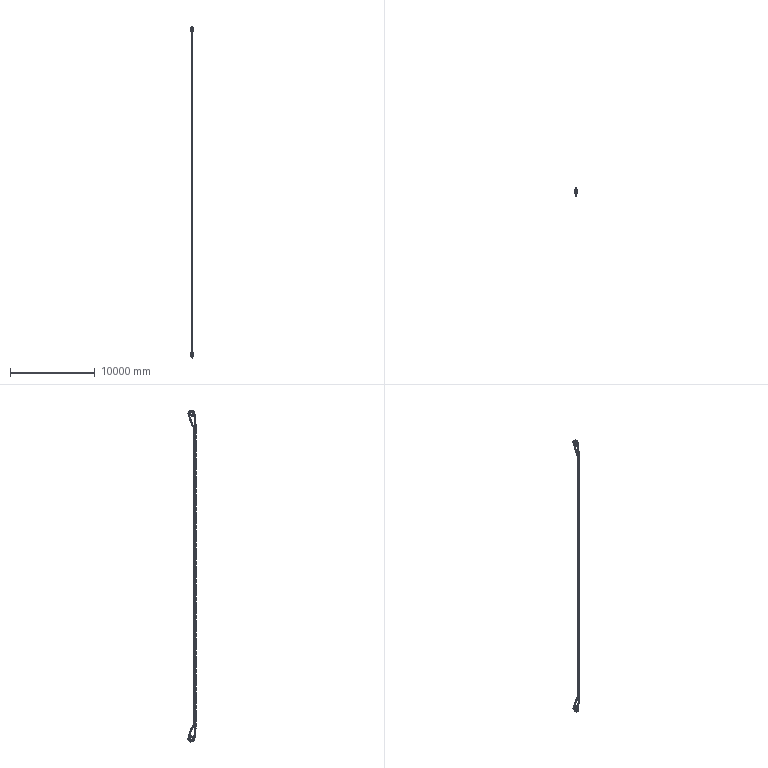Part | SolidWorks | features ReferencePattern 518, RefAxis 2, LocalChainPattern 1 | 522 solids | 6312 faces | volume 584235551 mm3 | torus 3152 | cylinder 2472 | spline 456 | plane 232 | commonest cylinder face diameters 48 x2144 285.1 x116 297.5 x116 604.088 x56 781 x28 420 x8